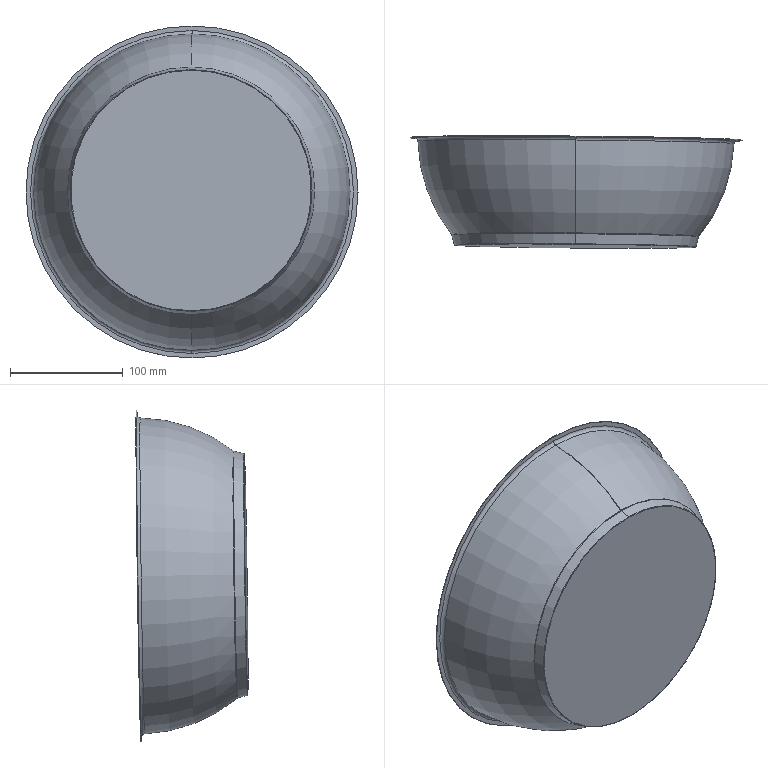Part | SolidWorks | features BaseBody 1 | 1 solid | 18 faces | box 294.994 x 99.661 x 294.977 mm | volume 413449 mm3 | torus 10 | plane 4 | cylinder 2 | cone 2 | commonest cylinder face diameters 295 x2
STEP:
#1=CARTESIAN_POINT('',(141.849,217.337,248.569));
#2=VERTEX_POINT('',#1);
#3=CARTESIAN_POINT('',(141.809,213.358,-32.392));
#4=VERTEX_POINT('',#3);
#5=CARTESIAN_POINT('',(141.829,215.348,108.088));
#6=DIRECTION('',(-0.008279,-0.9999,0.01416));
#7=DIRECTION('',(0.0001428,0.01416,0.9999));
#8=AXIS2_PLACEMENT_3D('',#5,#6,#7);
#9=CIRCLE('',#8,140.495);
#10=EDGE_CURVE('',#2,#4,#9,.T.);
#11=ORIENTED_EDGE('',*,*,#10,.F.);
#12=CARTESIAN_POINT('',(141.845,216.837,248.076));
#13=VERTEX_POINT('',#12);
#14=CARTESIAN_POINT('',(141.845,216.837,248.576));
#15=DIRECTION('',(-1.,0.00828,0.00002558));
#16=DIRECTION('',(-0.00828,-1.,0.));
#17=AXIS2_PLACEMENT_3D('',#14,#15,#16);
#18=CIRCLE('',#17,0.5);
#19=EDGE_CURVE('',#2,#13,#18,.T.);
#20=ORIENTED_EDGE('',*,*,#19,.T.);
#21=CARTESIAN_POINT('',(141.825,216.837,248.076));
#22=VERTEX_POINT('',#21);
#23=CARTESIAN_POINT('',(141.825,214.854,108.095));
#24=DIRECTION('',(0.008279,0.9999,-0.01416));
#25=DIRECTION('',(-0.0001428,-0.01416,-0.9999));
#26=AXIS2_PLACEMENT_3D('',#23,#24,#25);
#27=CIRCLE('',#26,139.995);
#28=EDGE_CURVE('',#22,#13,#27,.T.);
#29=ORIENTED_EDGE('',*,*,#28,.F.);
#30=CARTESIAN_POINT('',(141.805,212.872,-31.886));
#31=VERTEX_POINT('',#30);
#32=CARTESIAN_POINT('',(141.825,214.854,108.095));
#33=DIRECTION('',(0.008279,0.9999,-0.01416));
#34=DIRECTION('',(-0.0001428,-0.01416,-0.9999));
#35=AXIS2_PLACEMENT_3D('',#32,#33,#34);
#36=CIRCLE('',#35,139.995);
#37=EDGE_CURVE('',#31,#22,#36,.T.);
#38=ORIENTED_EDGE('',*,*,#37,.F.);
#39=CARTESIAN_POINT('',(141.804,212.858,-32.385));
#40=DIRECTION('',(1.,-0.00828,-0.00002558));
#41=DIRECTION('',(0.00828,1.,0.));
#42=AXIS2_PLACEMENT_3D('',#39,#40,#41);
#43=CIRCLE('',#42,0.5);
#44=EDGE_CURVE('',#4,#31,#43,.T.);
#45=ORIENTED_EDGE('',*,*,#44,.F.);
#46=EDGE_LOOP('',(#11,#20,#29,#38,#45));
#47=FACE_OUTER_BOUND('',#46,.T.);
#48=CARTESIAN_POINT('',(141.825,214.848,108.095));
#49=DIRECTION('',(0.008279,0.9999,-0.01416));
#50=DIRECTION('',(-0.0001428,-0.01416,-0.9999));
#51=AXIS2_PLACEMENT_3D('',#48,#49,#50);
#52=TOROIDAL_SURFACE('',#51,140.495,0.5);
#53=ADVANCED_FACE('',(#47),#52,.T.);
#54=CARTESIAN_POINT('',(141.825,212.872,-31.886));
#55=VERTEX_POINT('',#54);
#56=CARTESIAN_POINT('',(141.825,214.854,108.095));
#57=DIRECTION('',(0.008279,0.9999,-0.01416));
#58=DIRECTION('',(-0.0001428,-0.01416,-0.9999));
#59=AXIS2_PLACEMENT_3D('',#56,#57,#58);
#60=CIRCLE('',#59,139.995);
#61=EDGE_CURVE('',#55,#31,#60,.T.);
#62=ORIENTED_EDGE('',*,*,#61,.T.);
#63=ORIENTED_EDGE('',*,*,#37,.T.);
#64=CARTESIAN_POINT('',(141.121,131.414,219.047));
#65=VERTEX_POINT('',#64);
#66=CARTESIAN_POINT('',(141.839,216.596,108.576));
#67=DIRECTION('',(1.,-0.008278,0.0001172));
#68=DIRECTION('',(0.008278,1.,0.));
#69=AXIS2_PLACEMENT_3D('',#66,#67,#68);
#70=CIRCLE('',#69,139.5);
#71=EDGE_CURVE('',#22,#65,#70,.T.);
#72=ORIENTED_EDGE('',*,*,#71,.T.);
#73=CARTESIAN_POINT('',(141.121,128.305,-0.4489));
#74=VERTEX_POINT('',#73);
#75=CARTESIAN_POINT('',(141.121,129.859,109.299));
#76=DIRECTION('',(0.008279,0.9999,-0.01416));
#77=DIRECTION('',(0.,-0.01416,-0.9999));
#78=AXIS2_PLACEMENT_3D('',#75,#76,#77);
#79=CIRCLE('',#78,109.759);
#80=EDGE_CURVE('',#74,#65,#79,.T.);
#81=ORIENTED_EDGE('',*,*,#80,.F.);
#82=CARTESIAN_POINT('',(141.839,216.581,107.565));
#83=DIRECTION('',(-1.,0.008278,-0.0001172));
#84=DIRECTION('',(-0.008278,-1.,0.));
#85=AXIS2_PLACEMENT_3D('',#82,#83,#84);
#86=CIRCLE('',#85,139.5);
#87=EDGE_CURVE('',#55,#74,#86,.T.);
#88=ORIENTED_EDGE('',*,*,#87,.F.);
#89=EDGE_LOOP('',(#62,#63,#72,#81,#88));
#90=FACE_OUTER_BOUND('',#89,.T.);
#91=CARTESIAN_POINT('',(141.839,216.589,108.071));
#92=DIRECTION('',(-0.008279,-0.9999,0.01416));
#93=DIRECTION('',(0.,-0.01416,-0.9999));
#94=AXIS2_PLACEMENT_3D('',#91,#92,#93);
#95=TOROIDAL_SURFACE('',#94,0.5055,139.5);
#96=ADVANCED_FACE('',(#90),#95,.F.);
#97=CARTESIAN_POINT('',(141.846,216.937,255.58));
#98=VERTEX_POINT('',#97);
#99=CARTESIAN_POINT('',(141.803,212.759,-39.39));
#100=VERTEX_POINT('',#99);
#101=CARTESIAN_POINT('',(141.825,214.848,108.095));
#102=DIRECTION('',(-0.008279,-0.9999,0.01416));
#103=DIRECTION('',(0.0001428,0.01416,0.9999));
#104=AXIS2_PLACEMENT_3D('',#101,#102,#103);
#105=CIRCLE('',#104,147.5);
#106=EDGE_CURVE('',#98,#100,#105,.T.);
#107=ORIENTED_EDGE('',*,*,#106,.F.);
#108=CARTESIAN_POINT('',(141.85,217.437,255.573));
#109=VERTEX_POINT('',#108);
#110=CARTESIAN_POINT('',(141.85,217.437,255.573));
#111=DIRECTION('',(0.008279,0.9999,-0.01416));
#112=VECTOR('',#111,1000.);
#113=LINE('',#110,#112);
#114=EDGE_CURVE('',#98,#109,#113,.T.);
#115=ORIENTED_EDGE('',*,*,#114,.T.);
#116=CARTESIAN_POINT('',(141.808,213.259,-39.397));
#117=VERTEX_POINT('',#116);
#118=CARTESIAN_POINT('',(141.829,215.348,108.088));
#119=DIRECTION('',(0.008279,0.9999,-0.01416));
#120=DIRECTION('',(0.0001428,0.01416,0.9999));
#121=AXIS2_PLACEMENT_3D('',#118,#119,#120);
#122=CIRCLE('',#121,147.5);
#123=EDGE_CURVE('',#117,#109,#122,.T.);
#124=ORIENTED_EDGE('',*,*,#123,.F.);
#125=CARTESIAN_POINT('',(141.808,213.259,-39.397));
#126=DIRECTION('',(0.008279,0.9999,-0.01416));
#127=VECTOR('',#126,1000.);
#128=LINE('',#125,#127);
#129=EDGE_CURVE('',#100,#117,#128,.T.);
#130=ORIENTED_EDGE('',*,*,#129,.F.);
#131=EDGE_LOOP('',(#107,#115,#124,#130));
#132=FACE_OUTER_BOUND('',#131,.T.);
#133=CARTESIAN_POINT('',(141.829,215.348,108.088));
#134=DIRECTION('',(0.008279,0.9999,-0.01416));
#135=DIRECTION('',(-0.0001428,-0.01416,-0.9999));
#136=AXIS2_PLACEMENT_3D('',#133,#134,#135);
#137=CYLINDRICAL_SURFACE('',#136,147.5);
#138=ADVANCED_FACE('',(#132),#137,.T.);
#139=CARTESIAN_POINT('',(141.845,216.879,251.508));
#140=VERTEX_POINT('',#139);
#141=CARTESIAN_POINT('',(141.804,212.817,-35.317));
#142=VERTEX_POINT('',#141);
#143=CARTESIAN_POINT('',(141.825,214.848,108.095));
#144=DIRECTION('',(0.008279,0.9999,-0.01416));
#145=DIRECTION('',(0.0001428,0.01416,0.9999));
#146=AXIS2_PLACEMENT_3D('',#143,#144,#145);
#147=CIRCLE('',#146,143.427);
#148=EDGE_CURVE('',#140,#142,#147,.T.);
#149=ORIENTED_EDGE('',*,*,#148,.F.);
#150=CARTESIAN_POINT('',(141.821,213.936,248.551));
#151=VERTEX_POINT('',#150);
#152=CARTESIAN_POINT('',(141.82,213.879,251.55));
#153=DIRECTION('',(-1.,0.00828,0.00002558));
#154=DIRECTION('',(-0.00828,-1.,0.));
#155=AXIS2_PLACEMENT_3D('',#152,#153,#154);
#156=CIRCLE('',#155,3.);
#157=EDGE_CURVE('',#140,#151,#156,.T.);
#158=ORIENTED_EDGE('',*,*,#157,.T.);
#159=CARTESIAN_POINT('',(141.8,209.959,-32.278));
#160=VERTEX_POINT('',#159);
#161=CARTESIAN_POINT('',(141.8,211.948,108.136));
#162=DIRECTION('',(-0.008279,-0.9999,0.01416));
#163=DIRECTION('',(-0.0001428,-0.01416,-0.9999));
#164=AXIS2_PLACEMENT_3D('',#161,#162,#163);
#165=CIRCLE('',#164,140.429);
#166=EDGE_CURVE('',#160,#151,#165,.T.);
#167=ORIENTED_EDGE('',*,*,#166,.F.);
#168=CARTESIAN_POINT('',(141.78,209.959,-32.278));
#169=VERTEX_POINT('',#168);
#170=CARTESIAN_POINT('',(141.8,211.948,108.136));
#171=DIRECTION('',(-0.008279,-0.9999,0.01416));
#172=DIRECTION('',(-0.0001428,-0.01416,-0.9999));
#173=AXIS2_PLACEMENT_3D('',#170,#171,#172);
#174=CIRCLE('',#173,140.429);
#175=EDGE_CURVE('',#169,#160,#174,.T.);
#176=ORIENTED_EDGE('',*,*,#175,.F.);
#177=CARTESIAN_POINT('',(141.779,209.817,-35.275));
#178=DIRECTION('',(1.,-0.00828,-0.00002558));
#179=DIRECTION('',(0.00828,1.,0.));
#180=AXIS2_PLACEMENT_3D('',#177,#178,#179);
#181=CIRCLE('',#180,3.);
#182=EDGE_CURVE('',#142,#169,#181,.T.);
#183=ORIENTED_EDGE('',*,*,#182,.F.);
#184=EDGE_LOOP('',(#149,#158,#167,#176,#183));
#185=FACE_OUTER_BOUND('',#184,.T.);
#186=CARTESIAN_POINT('',(141.8,211.848,108.138));
#187=DIRECTION('',(0.008279,0.9999,-0.01416));
#188=DIRECTION('',(-0.0001428,-0.01416,-0.9999));
#189=AXIS2_PLACEMENT_3D('',#186,#187,#188);
#190=TOROIDAL_SURFACE('',#189,143.427,3.);
#191=ADVANCED_FACE('',(#185),#190,.F.);
#192=CARTESIAN_POINT('',(141.13,130.662,219.097));
#193=VERTEX_POINT('',#192);
#194=CARTESIAN_POINT('',(141.115,127.552,-0.4778));
#195=VERTEX_POINT('',#194);
#196=CARTESIAN_POINT('',(141.115,129.107,109.31));
#197=DIRECTION('',(0.008279,0.9999,-0.01416));
#198=DIRECTION('',(0.0001428,0.01416,0.9999));
#199=AXIS2_PLACEMENT_3D('',#196,#197,#198);
#200=CIRCLE('',#199,109.798);
#201=EDGE_CURVE('',#193,#195,#200,.T.);
#202=ORIENTED_EDGE('',*,*,#201,.T.);
#203=CARTESIAN_POINT('',(141.839,216.581,107.565));
#204=DIRECTION('',(1.,-0.008278,0.0001172));
#205=DIRECTION('',(0.008278,1.,0.));
#206=AXIS2_PLACEMENT_3D('',#203,#204,#205);
#207=CIRCLE('',#206,140.);
#208=EDGE_CURVE('',#195,#160,#207,.T.);
#209=ORIENTED_EDGE('',*,*,#208,.T.);
#210=ORIENTED_EDGE('',*,*,#166,.T.);
#211=CARTESIAN_POINT('',(141.8,213.937,248.551));
#212=VERTEX_POINT('',#211);
#213=CARTESIAN_POINT('',(141.8,211.948,108.136));
#214=DIRECTION('',(-0.008279,-0.9999,0.01416));
#215=DIRECTION('',(-0.0001428,-0.01416,-0.9999));
#216=AXIS2_PLACEMENT_3D('',#213,#214,#215);
#217=CIRCLE('',#216,140.429);
#218=EDGE_CURVE('',#151,#212,#217,.T.);
#219=ORIENTED_EDGE('',*,*,#218,.T.);
#220=CARTESIAN_POINT('',(141.115,130.662,219.097));
#221=VERTEX_POINT('',#220);
#222=CARTESIAN_POINT('',(141.839,216.596,108.576));
#223=DIRECTION('',(-1.,0.008278,-0.0001172));
#224=DIRECTION('',(-0.008278,-1.,0.));
#225=AXIS2_PLACEMENT_3D('',#222,#223,#224);
#226=CIRCLE('',#225,140.);
#227=EDGE_CURVE('',#221,#212,#226,.T.);
#228=ORIENTED_EDGE('',*,*,#227,.F.);
#229=CARTESIAN_POINT('',(141.115,129.107,109.31));
#230=DIRECTION('',(0.008279,0.9999,-0.01416));
#231=DIRECTION('',(0.0001428,0.01416,0.9999));
#232=AXIS2_PLACEMENT_3D('',#229,#230,#231);
#233=CIRCLE('',#232,109.798);
#234=EDGE_CURVE('',#221,#193,#233,.T.);
#235=ORIENTED_EDGE('',*,*,#234,.T.);
#236=EDGE_LOOP('',(#202,#209,#210,#219,#228,#235));
#237=FACE_OUTER_BOUND('',#236,.T.);
#238=CARTESIAN_POINT('',(141.839,216.589,108.071));
#239=DIRECTION('',(0.008279,0.9999,-0.01416));
#240=DIRECTION('',(0.,0.01416,0.9999));
#241=AXIS2_PLACEMENT_3D('',#238,#239,#240);
#242=TOROIDAL_SURFACE('',#241,0.5055,140.);
#243=ADVANCED_FACE('',(#237),#242,.T.);
#244=CARTESIAN_POINT('',(141.056,121.752,216.844));
#245=VERTEX_POINT('',#244);
#246=CARTESIAN_POINT('',(141.026,118.71,2.026));
#247=VERTEX_POINT('',#246);
#248=CARTESIAN_POINT('',(141.041,120.231,109.435));
#249=DIRECTION('',(-0.008279,-0.9999,0.01416));
#250=DIRECTION('',(0.0001428,0.01416,0.9999));
#251=AXIS2_PLACEMENT_3D('',#248,#249,#250);
#252=CIRCLE('',#251,107.42);
#253=EDGE_CURVE('',#245,#247,#252,.T.);
#254=ORIENTED_EDGE('',*,*,#253,.F.);
#255=CARTESIAN_POINT('',(141.093,126.207,217.971));
#256=DIRECTION('',(0.008034,0.9695,0.2451));
#257=VECTOR('',#256,1000.);
#258=LINE('',#255,#257);
#259=EDGE_CURVE('',#245,#193,#258,.T.);
#260=ORIENTED_EDGE('',*,*,#259,.T.);
#261=ORIENTED_EDGE('',*,*,#234,.F.);
#262=CARTESIAN_POINT('',(141.099,127.552,-0.4778));
#263=VERTEX_POINT('',#262);
#264=CARTESIAN_POINT('',(141.115,129.107,109.31));
#265=DIRECTION('',(0.008279,0.9999,-0.01416));
#266=DIRECTION('',(0.0001428,0.01416,0.9999));
#267=AXIS2_PLACEMENT_3D('',#264,#265,#266);
#268=CIRCLE('',#267,109.798);
#269=EDGE_CURVE('',#263,#221,#268,.T.);
#270=ORIENTED_EDGE('',*,*,#269,.F.);
#271=CARTESIAN_POINT('',(141.062,123.131,0.7742));
#272=DIRECTION('',(0.00796,0.9621,-0.2725));
#273=VECTOR('',#272,1000.);
#274=LINE('',#271,#273);
#275=EDGE_CURVE('',#247,#263,#274,.T.);
#276=ORIENTED_EDGE('',*,*,#275,.F.);
#277=EDGE_LOOP('',(#254,#260,#261,#270,#276));
#278=FACE_OUTER_BOUND('',#277,.T.);
#279=CARTESIAN_POINT('',(141.078,124.669,109.372));
#280=DIRECTION('',(0.008279,0.9999,-0.01416));
#281=DIRECTION('',(-0.0001428,-0.01416,-0.9999));
#282=AXIS2_PLACEMENT_3D('',#279,#280,#281);
#283=CONICAL_SURFACE('',#282,108.609,0.2618);
#284=ADVANCED_FACE('',(#278),#283,.T.);
#285=ORIENTED_EDGE('',*,*,#253,.T.);
#286=CARTESIAN_POINT('',(141.023,118.346,2.514));
#287=VERTEX_POINT('',#286);
#288=CARTESIAN_POINT('',(141.027,118.846,2.507));
#289=DIRECTION('',(-1.,0.00828,0.00002558));
#290=DIRECTION('',(-0.00828,-1.,0.));
#291=AXIS2_PLACEMENT_3D('',#288,#289,#290);
#292=CIRCLE('',#291,0.5);
#293=EDGE_CURVE('',#247,#287,#292,.T.);
#294=ORIENTED_EDGE('',*,*,#293,.T.);
#295=CARTESIAN_POINT('',(141.053,121.375,216.367));
#296=VERTEX_POINT('',#295);
#297=CARTESIAN_POINT('',(141.038,119.861,109.441));
#298=DIRECTION('',(-0.008279,-0.9999,0.01416));
#299=DIRECTION('',(-0.0001428,-0.01416,-0.9999));
#300=AXIS2_PLACEMENT_3D('',#297,#298,#299);
#301=CIRCLE('',#300,106.937);
#302=EDGE_CURVE('',#296,#287,#301,.T.);
#303=ORIENTED_EDGE('',*,*,#302,.F.);
#304=CARTESIAN_POINT('',(141.057,121.875,216.36));
#305=DIRECTION('',(1.,-0.00828,-0.00002558));
#306=DIRECTION('',(0.00828,1.,0.));
#307=AXIS2_PLACEMENT_3D('',#304,#305,#306);
#308=CIRCLE('',#307,0.5);
#309=EDGE_CURVE('',#245,#296,#308,.T.);
#310=ORIENTED_EDGE('',*,*,#309,.F.);
#311=EDGE_LOOP('',(#285,#294,#303,#310));
#312=FACE_OUTER_BOUND('',#311,.T.);
#313=CARTESIAN_POINT('',(141.042,120.361,109.433));
#314=DIRECTION('',(-0.008279,-0.9999,0.01416));
#315=DIRECTION('',(0.0001428,0.01416,0.9999));
#316=AXIS2_PLACEMENT_3D('',#313,#314,#315);
#317=TOROIDAL_SURFACE('',#316,106.937,0.5);
#318=ADVANCED_FACE('',(#312),#317,.T.);
#319=ORIENTED_EDGE('',*,*,#302,.T.);
#320=CARTESIAN_POINT('',(141.038,119.861,109.441));
#321=DIRECTION('',(-0.008279,-0.9999,0.01416));
#322=DIRECTION('',(-0.0001428,-0.01416,-0.9999));
#323=AXIS2_PLACEMENT_3D('',#320,#321,#322);
#324=CIRCLE('',#323,106.937);
#325=EDGE_CURVE('',#287,#296,#324,.T.);
#326=ORIENTED_EDGE('',*,*,#325,.T.);
#327=EDGE_LOOP('',(#319,#326));
#328=FACE_OUTER_BOUND('',#327,.T.);
#329=CARTESIAN_POINT('',(141.038,119.861,109.441));
#330=DIRECTION('',(-0.008279,-0.9999,0.01416));
#331=DIRECTION('',(-1.,0.00828,0.));
#332=AXIS2_PLACEMENT_3D('',#329,#330,#331);
#333=PLANE('',#332);
#334=ADVANCED_FACE('',(#328),#333,.T.);
#335=ORIENTED_EDGE('',*,*,#293,.F.);
#336=CARTESIAN_POINT('',(141.041,120.231,109.435));
#337=DIRECTION('',(-0.008279,-0.9999,0.01416));
#338=DIRECTION('',(0.0001428,0.01416,0.9999));
#339=AXIS2_PLACEMENT_3D('',#336,#337,#338);
#340=CIRCLE('',#339,107.42);
#341=EDGE_CURVE('',#247,#245,#340,.T.);
#342=ORIENTED_EDGE('',*,*,#341,.T.);
#343=ORIENTED_EDGE('',*,*,#309,.T.);
#344=ORIENTED_EDGE('',*,*,#325,.F.);
#345=EDGE_LOOP('',(#335,#342,#343,#344));
#346=FACE_OUTER_BOUND('',#345,.T.);
#347=CARTESIAN_POINT('',(141.042,120.361,109.433));
#348=DIRECTION('',(-0.008279,-0.9999,0.01416));
#349=DIRECTION('',(0.0001428,0.01416,0.9999));
#350=AXIS2_PLACEMENT_3D('',#347,#348,#349);
#351=TOROIDAL_SURFACE('',#350,106.937,0.5);
#352=ADVANCED_FACE('',(#346),#351,.T.);
#353=ORIENTED_EDGE('',*,*,#259,.F.);
#354=ORIENTED_EDGE('',*,*,#341,.F.);
#355=ORIENTED_EDGE('',*,*,#275,.T.);
#356=CARTESIAN_POINT('',(141.115,129.107,109.31));
#357=DIRECTION('',(0.008279,0.9999,-0.01416));
#358=DIRECTION('',(0.0001428,0.01416,0.9999));
#359=AXIS2_PLACEMENT_3D('',#356,#357,#358);
#360=CIRCLE('',#359,109.798);
#361=EDGE_CURVE('',#195,#263,#360,.T.);
#362=ORIENTED_EDGE('',*,*,#361,.F.);
#363=ORIENTED_EDGE('',*,*,#201,.F.);
#364=EDGE_LOOP('',(#353,#354,#355,#362,#363));
#365=FACE_OUTER_BOUND('',#364,.T.);
#366=CARTESIAN_POINT('',(141.078,124.669,109.372));
#367=DIRECTION('',(0.008279,0.9999,-0.01416));
#368=DIRECTION('',(-0.0001428,-0.01416,-0.9999));
#369=AXIS2_PLACEMENT_3D('',#366,#367,#368);
#370=CONICAL_SURFACE('',#369,108.609,0.2618);
#371=ADVANCED_FACE('',(#365),#370,.T.);
#372=ORIENTED_EDGE('',*,*,#208,.F.);
#373=ORIENTED_EDGE('',*,*,#361,.T.);
#374=ORIENTED_EDGE('',*,*,#269,.T.);
#375=ORIENTED_EDGE('',*,*,#227,.T.);
#376=CARTESIAN_POINT('',(141.8,211.948,108.136));
#377=DIRECTION('',(-0.008279,-0.9999,0.01416));
#378=DIRECTION('',(-0.0001428,-0.01416,-0.9999));
#379=AXIS2_PLACEMENT_3D('',#376,#377,#378);
#380=CIRCLE('',#379,140.429);
#381=EDGE_CURVE('',#212,#169,#380,.T.);
#382=ORIENTED_EDGE('',*,*,#381,.T.);
#383=ORIENTED_EDGE('',*,*,#175,.T.);
#384=EDGE_LOOP('',(#372,#373,#374,#375,#382,#383));
#385=FACE_OUTER_BOUND('',#384,.T.);
#386=CARTESIAN_POINT('',(141.839,216.589,108.071));
#387=DIRECTION('',(0.008279,0.9999,-0.01416));
#388=DIRECTION('',(0.,0.01416,0.9999));
#389=AXIS2_PLACEMENT_3D('',#386,#387,#388);
#390=TOROIDAL_SURFACE('',#389,0.5055,140.);
#391=ADVANCED_FACE('',(#385),#390,.T.);
#392=ORIENTED_EDGE('',*,*,#157,.F.);
#393=CARTESIAN_POINT('',(141.825,214.848,108.095));
#394=DIRECTION('',(0.008279,0.9999,-0.01416));
#395=DIRECTION('',(0.0001428,0.01416,0.9999));
#396=AXIS2_PLACEMENT_3D('',#393,#394,#395);
#397=CIRCLE('',#396,143.427);
#398=EDGE_CURVE('',#142,#140,#397,.T.);
#399=ORIENTED_EDGE('',*,*,#398,.F.);
#400=ORIENTED_EDGE('',*,*,#182,.T.);
#401=ORIENTED_EDGE('',*,*,#381,.F.);
#402=ORIENTED_EDGE('',*,*,#218,.F.);
#403=EDGE_LOOP('',(#392,#399,#400,#401,#402));
#404=FACE_OUTER_BOUND('',#403,.T.);
#405=CARTESIAN_POINT('',(141.8,211.848,108.138));
#406=DIRECTION('',(0.008279,0.9999,-0.01416));
#407=DIRECTION('',(-0.0001428,-0.01416,-0.9999));
#408=AXIS2_PLACEMENT_3D('',#405,#406,#407);
#409=TOROIDAL_SURFACE('',#408,143.427,3.);
#410=ADVANCED_FACE('',(#404),#409,.F.);
#411=ORIENTED_EDGE('',*,*,#398,.T.);
#412=ORIENTED_EDGE('',*,*,#148,.T.);
#413=EDGE_LOOP('',(#411,#412));
#414=FACE_BOUND('',#413,.T.);
#415=CARTESIAN_POINT('',(141.825,214.848,108.095));
#416=DIRECTION('',(-0.008279,-0.9999,0.01416));
#417=DIRECTION('',(0.0001428,0.01416,0.9999));
#418=AXIS2_PLACEMENT_3D('',#415,#416,#417);
#419=CIRCLE('',#418,147.5);
#420=EDGE_CURVE('',#100,#98,#419,.T.);
#421=ORIENTED_EDGE('',*,*,#420,.T.);
#422=ORIENTED_EDGE('',*,*,#106,.T.);
#423=EDGE_LOOP('',(#421,#422));
#424=FACE_OUTER_BOUND('',#423,.T.);
#425=CARTESIAN_POINT('',(-5.67,216.069,108.099));
#426=DIRECTION('',(0.008279,0.9999,-0.01416));
#427=DIRECTION('',(-0.8633,0.,-0.5047));
#428=AXIS2_PLACEMENT_3D('',#425,#426,#427);
#429=PLANE('',#428);
#430=ADVANCED_FACE('',(#414,#424),#429,.F.);
#431=ORIENTED_EDGE('',*,*,#114,.F.);
#432=ORIENTED_EDGE('',*,*,#420,.F.);
#433=ORIENTED_EDGE('',*,*,#129,.T.);
#434=CARTESIAN_POINT('',(141.829,215.348,108.088));
#435=DIRECTION('',(0.008279,0.9999,-0.01416));
#436=DIRECTION('',(0.0001428,0.01416,0.9999));
#437=AXIS2_PLACEMENT_3D('',#434,#435,#436);
#438=CIRCLE('',#437,147.5);
#439=EDGE_CURVE('',#109,#117,#438,.T.);
#440=ORIENTED_EDGE('',*,*,#439,.F.);
#441=EDGE_LOOP('',(#431,#432,#433,#440));
#442=FACE_OUTER_BOUND('',#441,.T.);
#443=CARTESIAN_POINT('',(141.829,215.348,108.088));
#444=DIRECTION('',(0.008279,0.9999,-0.01416));
#445=DIRECTION('',(-0.0001428,-0.01416,-0.9999));
#446=AXIS2_PLACEMENT_3D('',#443,#444,#445);
#447=CYLINDRICAL_SURFACE('',#446,147.5);
#448=ADVANCED_FACE('',(#442),#447,.T.);
#449=ORIENTED_EDGE('',*,*,#80,.T.);
#450=CARTESIAN_POINT('',(141.121,129.859,109.299));
#451=DIRECTION('',(0.008279,0.9999,-0.01416));
#452=DIRECTION('',(0.,-0.01416,-0.9999));
#453=AXIS2_PLACEMENT_3D('',#450,#451,#452);
#454=CIRCLE('',#453,109.759);
#455=EDGE_CURVE('',#65,#74,#454,.T.);
#456=ORIENTED_EDGE('',*,*,#455,.T.);
#457=EDGE_LOOP('',(#449,#456));
#458=FACE_OUTER_BOUND('',#457,.T.);
#459=CARTESIAN_POINT('',(141.121,129.859,109.299));
#460=DIRECTION('',(-0.008279,-0.9999,0.01416));
#461=DIRECTION('',(-1.,0.00828,0.));
#462=AXIS2_PLACEMENT_3D('',#459,#460,#461);
#463=PLANE('',#462);
#464=ADVANCED_FACE('',(#458),#463,.F.);
#465=ORIENTED_EDGE('',*,*,#71,.F.);
#466=ORIENTED_EDGE('',*,*,#28,.T.);
#467=CARTESIAN_POINT('',(141.825,214.854,108.095));
#468=DIRECTION('',(0.008279,0.9999,-0.01416));
#469=DIRECTION('',(-0.0001428,-0.01416,-0.9999));
#470=AXIS2_PLACEMENT_3D('',#467,#468,#469);
#471=CIRCLE('',#470,139.995);
#472=EDGE_CURVE('',#13,#55,#471,.T.);
#473=ORIENTED_EDGE('',*,*,#472,.T.);
#474=ORIENTED_EDGE('',*,*,#87,.T.);
#475=ORIENTED_EDGE('',*,*,#455,.F.);
#476=EDGE_LOOP('',(#465,#466,#473,#474,#475));
#477=FACE_OUTER_BOUND('',#476,.T.);
#478=CARTESIAN_POINT('',(141.839,216.589,108.071));
#479=DIRECTION('',(-0.008279,-0.9999,0.01416));
#480=DIRECTION('',(0.,-0.01416,-0.9999));
#481=AXIS2_PLACEMENT_3D('',#478,#479,#480);
#482=TOROIDAL_SURFACE('',#481,0.5055,139.5);
#483=ADVANCED_FACE('',(#477),#482,.F.);
#484=ORIENTED_EDGE('',*,*,#19,.F.);
#485=CARTESIAN_POINT('',(141.829,215.348,108.088));
#486=DIRECTION('',(-0.008279,-0.9999,0.01416));
#487=DIRECTION('',(0.0001428,0.01416,0.9999));
#488=AXIS2_PLACEMENT_3D('',#485,#486,#487);
#489=CIRCLE('',#488,140.495);
#490=EDGE_CURVE('',#4,#2,#489,.T.);
#491=ORIENTED_EDGE('',*,*,#490,.F.);
#492=ORIENTED_EDGE('',*,*,#44,.T.);
#493=ORIENTED_EDGE('',*,*,#61,.F.);
#494=ORIENTED_EDGE('',*,*,#472,.F.);
#495=EDGE_LOOP('',(#484,#491,#492,#493,#494));
#496=FACE_OUTER_BOUND('',#495,.T.);
#497=CARTESIAN_POINT('',(141.825,214.848,108.095));
#498=DIRECTION('',(0.008279,0.9999,-0.01416));
#499=DIRECTION('',(-0.0001428,-0.01416,-0.9999));
#500=AXIS2_PLACEMENT_3D('',#497,#498,#499);
#501=TOROIDAL_SURFACE('',#500,140.495,0.5);
#502=ADVANCED_FACE('',(#496),#501,.T.);
#503=ORIENTED_EDGE('',*,*,#490,.T.);
#504=ORIENTED_EDGE('',*,*,#10,.T.);
#505=EDGE_LOOP('',(#503,#504));
#506=FACE_BOUND('',#505,.T.);
#507=ORIENTED_EDGE('',*,*,#123,.T.);
#508=ORIENTED_EDGE('',*,*,#439,.T.);
#509=EDGE_LOOP('',(#507,#508));
#510=FACE_OUTER_BOUND('',#509,.T.);
#511=CARTESIAN_POINT('',(141.829,215.348,108.088));
#512=DIRECTION('',(0.008279,0.9999,-0.01416));
#513=DIRECTION('',(-0.8633,0.,-0.5047));
#514=AXIS2_PLACEMENT_3D('',#511,#512,#513);
#515=PLANE('',#514);
#516=ADVANCED_FACE('',(#506,#510),#515,.T.);
#517=CLOSED_SHELL('',(#53,#96,#138,#191,#243,#284,#318,#334,#352,#371,#391,#410,#430,#448,#464,#483,#502,#516));
#518=MANIFOLD_SOLID_BREP('',#517);
#519=CARTESIAN_POINT('',(0.,0.,0.));
#520=DIRECTION('',(0.,0.,1.));
#521=DIRECTION('',(1.,0.,0.));
#522=AXIS2_PLACEMENT_3D('',#519,#520,#521);
#523=(LENGTH_UNIT()NAMED_UNIT(*)SI_UNIT(.MILLI.,.METRE.));
#524=UNCERTAINTY_MEASURE_WITH_UNIT(LENGTH_MEASURE(0.00001),#523,'','');
#525=(NAMED_UNIT(*)PLANE_ANGLE_UNIT()SI_UNIT($,.RADIAN.));
#526=(NAMED_UNIT(*)SI_UNIT($,.STERADIAN.)SOLID_ANGLE_UNIT());
#527=(GEOMETRIC_REPRESENTATION_CONTEXT(3)GLOBAL_UNCERTAINTY_ASSIGNED_CONTEXT((#524))GLOBAL_UNIT_ASSIGNED_CONTEXT((#523,#525,#526))REPRESENTATION_CONTEXT('',''));
#528=ADVANCED_BREP_SHAPE_REPRESENTATION('',(#518,#522),#527);